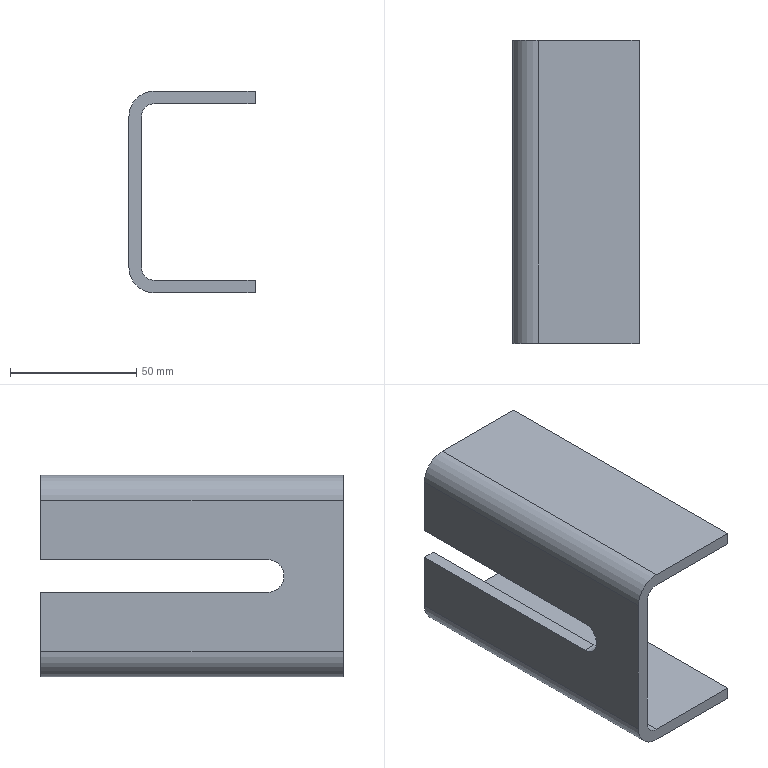Part | SolidWorks | features BaseBody 1 | 1 solid | 18 faces | box 50 x 120 x 80 mm | volume 91955 mm3 | plane 13 | cylinder 5 | commonest cylinder face diameters 10 x2 20 x2 13 x1
STEP:
#1=CARTESIAN_POINT('',(-50.,120.,21.101));
#2=VERTEX_POINT('',#1);
#3=CARTESIAN_POINT('',(-50.,30.,21.101));
#4=VERTEX_POINT('',#3);
#5=CARTESIAN_POINT('',(-50.,60.,21.101));
#6=DIRECTION('',(0.,-1.,0.));
#7=VECTOR('',#6,1000.);
#8=LINE('',#5,#7);
#9=EDGE_CURVE('',#2,#4,#8,.T.);
#10=ORIENTED_EDGE('',*,*,#9,.T.);
#11=CARTESIAN_POINT('',(-50.,30.,8.101));
#12=VERTEX_POINT('',#11);
#13=CARTESIAN_POINT('',(-50.,30.,14.601));
#14=DIRECTION('',(1.,0.,0.));
#15=DIRECTION('',(0.,0.,-1.));
#16=AXIS2_PLACEMENT_3D('',#13,#14,#15);
#17=CIRCLE('',#16,6.5);
#18=EDGE_CURVE('',#4,#12,#17,.T.);
#19=ORIENTED_EDGE('',*,*,#18,.T.);
#20=CARTESIAN_POINT('',(-50.,120.,8.101));
#21=VERTEX_POINT('',#20);
#22=CARTESIAN_POINT('',(-50.,60.,8.101));
#23=DIRECTION('',(0.,1.,0.));
#24=VECTOR('',#23,1000.);
#25=LINE('',#22,#24);
#26=EDGE_CURVE('',#12,#21,#25,.T.);
#27=ORIENTED_EDGE('',*,*,#26,.T.);
#28=CARTESIAN_POINT('',(-50.,120.,-15.399));
#29=VERTEX_POINT('',#28);
#30=CARTESIAN_POINT('',(-50.,120.,14.601));
#31=DIRECTION('',(0.,0.,-1.));
#32=VECTOR('',#31,1000.);
#33=LINE('',#30,#32);
#34=EDGE_CURVE('',#21,#29,#33,.T.);
#35=ORIENTED_EDGE('',*,*,#34,.T.);
#36=CARTESIAN_POINT('',(-50.,0.,-15.399));
#37=VERTEX_POINT('',#36);
#38=CARTESIAN_POINT('',(-50.,60.,-15.399));
#39=DIRECTION('',(0.,-1.,0.));
#40=VECTOR('',#39,1000.);
#41=LINE('',#38,#40);
#42=EDGE_CURVE('',#29,#37,#41,.T.);
#43=ORIENTED_EDGE('',*,*,#42,.T.);
#44=CARTESIAN_POINT('',(-50.,0.,44.601));
#45=VERTEX_POINT('',#44);
#46=CARTESIAN_POINT('',(-50.,0.,14.601));
#47=DIRECTION('',(0.,0.,1.));
#48=VECTOR('',#47,1000.);
#49=LINE('',#46,#48);
#50=EDGE_CURVE('',#37,#45,#49,.T.);
#51=ORIENTED_EDGE('',*,*,#50,.T.);
#52=CARTESIAN_POINT('',(-50.,120.,44.601));
#53=VERTEX_POINT('',#52);
#54=CARTESIAN_POINT('',(-50.,60.,44.601));
#55=DIRECTION('',(0.,1.,0.));
#56=VECTOR('',#55,1000.);
#57=LINE('',#54,#56);
#58=EDGE_CURVE('',#45,#53,#57,.T.);
#59=ORIENTED_EDGE('',*,*,#58,.T.);
#60=CARTESIAN_POINT('',(-50.,120.,14.601));
#61=DIRECTION('',(0.,0.,-1.));
#62=VECTOR('',#61,1000.);
#63=LINE('',#60,#62);
#64=EDGE_CURVE('',#53,#2,#63,.T.);
#65=ORIENTED_EDGE('',*,*,#64,.T.);
#66=EDGE_LOOP('',(#10,#19,#27,#35,#43,#51,#59,#65));
#67=FACE_OUTER_BOUND('',#66,.T.);
#68=CARTESIAN_POINT('',(-50.,60.,14.601));
#69=DIRECTION('',(-1.,0.,0.));
#70=DIRECTION('',(0.,0.,1.));
#71=AXIS2_PLACEMENT_3D('',#68,#69,#70);
#72=PLANE('',#71);
#73=ADVANCED_FACE('',(#67),#72,.T.);
#74=CARTESIAN_POINT('',(-45.,30.,21.101));
#75=VERTEX_POINT('',#74);
#76=CARTESIAN_POINT('',(-50.,30.,21.101));
#77=DIRECTION('',(-1.,0.,0.));
#78=VECTOR('',#77,1000.);
#79=LINE('',#76,#78);
#80=EDGE_CURVE('',#75,#4,#79,.T.);
#81=ORIENTED_EDGE('',*,*,#80,.F.);
#82=CARTESIAN_POINT('',(-45.,30.,8.101));
#83=VERTEX_POINT('',#82);
#84=CARTESIAN_POINT('',(-45.,30.,14.601));
#85=DIRECTION('',(-1.,0.,0.));
#86=DIRECTION('',(0.,0.,-1.));
#87=AXIS2_PLACEMENT_3D('',#84,#85,#86);
#88=CIRCLE('',#87,6.5);
#89=EDGE_CURVE('',#83,#75,#88,.T.);
#90=ORIENTED_EDGE('',*,*,#89,.F.);
#91=CARTESIAN_POINT('',(-50.,30.,8.101));
#92=DIRECTION('',(1.,0.,0.));
#93=VECTOR('',#92,1000.);
#94=LINE('',#91,#93);
#95=EDGE_CURVE('',#12,#83,#94,.T.);
#96=ORIENTED_EDGE('',*,*,#95,.F.);
#97=ORIENTED_EDGE('',*,*,#18,.F.);
#98=EDGE_LOOP('',(#81,#90,#96,#97));
#99=FACE_OUTER_BOUND('',#98,.T.);
#100=CARTESIAN_POINT('',(-50.,30.,14.601));
#101=DIRECTION('',(1.,0.,0.));
#102=DIRECTION('',(0.,0.,-1.));
#103=AXIS2_PLACEMENT_3D('',#100,#101,#102);
#104=CYLINDRICAL_SURFACE('',#103,6.5);
#105=ADVANCED_FACE('',(#99),#104,.F.);
#106=CARTESIAN_POINT('',(-45.,120.,21.101));
#107=VERTEX_POINT('',#106);
#108=CARTESIAN_POINT('',(-50.,120.,21.101));
#109=DIRECTION('',(-1.,0.,0.));
#110=VECTOR('',#109,1000.);
#111=LINE('',#108,#110);
#112=EDGE_CURVE('',#107,#2,#111,.T.);
#113=ORIENTED_EDGE('',*,*,#112,.F.);
#114=CARTESIAN_POINT('',(-45.,120.,21.101));
#115=DIRECTION('',(0.,1.,0.));
#116=VECTOR('',#115,1000.);
#117=LINE('',#114,#116);
#118=EDGE_CURVE('',#75,#107,#117,.T.);
#119=ORIENTED_EDGE('',*,*,#118,.F.);
#120=ORIENTED_EDGE('',*,*,#80,.T.);
#121=ORIENTED_EDGE('',*,*,#9,.F.);
#122=EDGE_LOOP('',(#113,#119,#120,#121));
#123=FACE_OUTER_BOUND('',#122,.T.);
#124=CARTESIAN_POINT('',(-50.,120.,21.101));
#125=DIRECTION('',(0.,0.,1.));
#126=DIRECTION('',(0.,-1.,0.));
#127=AXIS2_PLACEMENT_3D('',#124,#125,#126);
#128=PLANE('',#127);
#129=ADVANCED_FACE('',(#123),#128,.F.);
#130=ORIENTED_EDGE('',*,*,#64,.F.);
#131=CARTESIAN_POINT('',(-40.,120.,54.601));
#132=VERTEX_POINT('',#131);
#133=CARTESIAN_POINT('',(-40.,120.,44.601));
#134=DIRECTION('',(0.,-1.,0.));
#135=DIRECTION('',(0.,0.,-1.));
#136=AXIS2_PLACEMENT_3D('',#133,#134,#135);
#137=CIRCLE('',#136,10.);
#138=EDGE_CURVE('',#132,#53,#137,.T.);
#139=ORIENTED_EDGE('',*,*,#138,.F.);
#140=CARTESIAN_POINT('',(0.,120.,54.601));
#141=VERTEX_POINT('',#140);
#142=CARTESIAN_POINT('',(-81.31,120.,54.601));
#143=DIRECTION('',(-1.,0.,0.));
#144=VECTOR('',#143,1000.);
#145=LINE('',#142,#144);
#146=EDGE_CURVE('',#141,#132,#145,.T.);
#147=ORIENTED_EDGE('',*,*,#146,.F.);
#148=CARTESIAN_POINT('',(0.,120.,49.601));
#149=VERTEX_POINT('',#148);
#150=CARTESIAN_POINT('',(0.,120.,49.601));
#151=DIRECTION('',(0.,0.,-1.));
#152=VECTOR('',#151,1000.);
#153=LINE('',#150,#152);
#154=EDGE_CURVE('',#141,#149,#153,.T.);
#155=ORIENTED_EDGE('',*,*,#154,.T.);
#156=CARTESIAN_POINT('',(-40.,120.,49.601));
#157=VERTEX_POINT('',#156);
#158=CARTESIAN_POINT('',(-40.,120.,49.601));
#159=DIRECTION('',(-1.,0.,0.));
#160=VECTOR('',#159,1000.);
#161=LINE('',#158,#160);
#162=EDGE_CURVE('',#149,#157,#161,.T.);
#163=ORIENTED_EDGE('',*,*,#162,.T.);
#164=CARTESIAN_POINT('',(-45.,120.,44.601));
#165=VERTEX_POINT('',#164);
#166=CARTESIAN_POINT('',(-40.,120.,44.601));
#167=DIRECTION('',(0.,-1.,0.));
#168=DIRECTION('',(0.,0.,-1.));
#169=AXIS2_PLACEMENT_3D('',#166,#167,#168);
#170=CIRCLE('',#169,5.);
#171=EDGE_CURVE('',#157,#165,#170,.T.);
#172=ORIENTED_EDGE('',*,*,#171,.T.);
#173=CARTESIAN_POINT('',(-45.,120.,55.911));
#174=DIRECTION('',(0.,0.,-1.));
#175=VECTOR('',#174,1000.);
#176=LINE('',#173,#175);
#177=EDGE_CURVE('',#165,#107,#176,.T.);
#178=ORIENTED_EDGE('',*,*,#177,.T.);
#179=ORIENTED_EDGE('',*,*,#112,.T.);
#180=EDGE_LOOP('',(#130,#139,#147,#155,#163,#172,#178,#179));
#181=FACE_OUTER_BOUND('',#180,.T.);
#182=CARTESIAN_POINT('',(-45.,120.,55.911));
#183=DIRECTION('',(0.,1.,0.));
#184=DIRECTION('',(0.,0.,1.));
#185=AXIS2_PLACEMENT_3D('',#182,#183,#184);
#186=PLANE('',#185);
#187=ADVANCED_FACE('',(#181),#186,.T.);
#188=CARTESIAN_POINT('',(-40.,0.,54.601));
#189=VERTEX_POINT('',#188);
#190=CARTESIAN_POINT('',(-40.,60.,54.601));
#191=DIRECTION('',(0.,1.,0.));
#192=VECTOR('',#191,1000.);
#193=LINE('',#190,#192);
#194=EDGE_CURVE('',#189,#132,#193,.T.);
#195=ORIENTED_EDGE('',*,*,#194,.T.);
#196=ORIENTED_EDGE('',*,*,#138,.T.);
#197=ORIENTED_EDGE('',*,*,#58,.F.);
#198=CARTESIAN_POINT('',(-40.,0.,44.601));
#199=DIRECTION('',(0.,1.,0.));
#200=DIRECTION('',(0.,0.,-1.));
#201=AXIS2_PLACEMENT_3D('',#198,#199,#200);
#202=CIRCLE('',#201,10.);
#203=EDGE_CURVE('',#45,#189,#202,.T.);
#204=ORIENTED_EDGE('',*,*,#203,.T.);
#205=EDGE_LOOP('',(#195,#196,#197,#204));
#206=FACE_OUTER_BOUND('',#205,.T.);
#207=CARTESIAN_POINT('',(-40.,60.,44.601));
#208=DIRECTION('',(0.,-1.,0.));
#209=DIRECTION('',(0.,0.,-1.));
#210=AXIS2_PLACEMENT_3D('',#207,#208,#209);
#211=CYLINDRICAL_SURFACE('',#210,10.);
#212=ADVANCED_FACE('',(#206),#211,.T.);
#213=CARTESIAN_POINT('',(-45.,0.,-15.399));
#214=VERTEX_POINT('',#213);
#215=CARTESIAN_POINT('',(-45.,0.,44.601));
#216=VERTEX_POINT('',#215);
#217=CARTESIAN_POINT('',(-45.,0.,-26.709));
#218=DIRECTION('',(0.,0.,1.));
#219=VECTOR('',#218,1000.);
#220=LINE('',#217,#219);
#221=EDGE_CURVE('',#214,#216,#220,.T.);
#222=ORIENTED_EDGE('',*,*,#221,.T.);
#223=CARTESIAN_POINT('',(-40.,0.,49.601));
#224=VERTEX_POINT('',#223);
#225=CARTESIAN_POINT('',(-40.,0.,44.601));
#226=DIRECTION('',(0.,1.,0.));
#227=DIRECTION('',(0.,0.,-1.));
#228=AXIS2_PLACEMENT_3D('',#225,#226,#227);
#229=CIRCLE('',#228,5.);
#230=EDGE_CURVE('',#216,#224,#229,.T.);
#231=ORIENTED_EDGE('',*,*,#230,.T.);
#232=CARTESIAN_POINT('',(0.,0.,49.601));
#233=VERTEX_POINT('',#232);
#234=CARTESIAN_POINT('',(-122.619,0.,49.601));
#235=DIRECTION('',(1.,0.,0.));
#236=VECTOR('',#235,1000.);
#237=LINE('',#234,#236);
#238=EDGE_CURVE('',#224,#233,#237,.T.);
#239=ORIENTED_EDGE('',*,*,#238,.T.);
#240=CARTESIAN_POINT('',(0.,0.,54.601));
#241=VERTEX_POINT('',#240);
#242=CARTESIAN_POINT('',(0.,0.,49.601));
#243=DIRECTION('',(0.,0.,-1.));
#244=VECTOR('',#243,1000.);
#245=LINE('',#242,#244);
#246=EDGE_CURVE('',#241,#233,#245,.T.);
#247=ORIENTED_EDGE('',*,*,#246,.F.);
#248=CARTESIAN_POINT('',(-81.31,0.,54.601));
#249=DIRECTION('',(1.,0.,0.));
#250=VECTOR('',#249,1000.);
#251=LINE('',#248,#250);
#252=EDGE_CURVE('',#189,#241,#251,.T.);
#253=ORIENTED_EDGE('',*,*,#252,.F.);
#254=ORIENTED_EDGE('',*,*,#203,.F.);
#255=ORIENTED_EDGE('',*,*,#50,.F.);
#256=CARTESIAN_POINT('',(-40.,0.,-25.399));
#257=VERTEX_POINT('',#256);
#258=CARTESIAN_POINT('',(-40.,0.,-15.399));
#259=DIRECTION('',(0.,1.,0.));
#260=DIRECTION('',(0.,0.,-1.));
#261=AXIS2_PLACEMENT_3D('',#258,#259,#260);
#262=CIRCLE('',#261,10.);
#263=EDGE_CURVE('',#257,#37,#262,.T.);
#264=ORIENTED_EDGE('',*,*,#263,.F.);
#265=CARTESIAN_POINT('',(0.,0.,-25.399));
#266=VERTEX_POINT('',#265);
#267=CARTESIAN_POINT('',(-81.31,0.,-25.399));
#268=DIRECTION('',(-1.,0.,0.));
#269=VECTOR('',#268,1000.);
#270=LINE('',#267,#269);
#271=EDGE_CURVE('',#266,#257,#270,.T.);
#272=ORIENTED_EDGE('',*,*,#271,.F.);
#273=CARTESIAN_POINT('',(0.,0.,-20.399));
#274=VERTEX_POINT('',#273);
#275=CARTESIAN_POINT('',(0.,0.,-20.399));
#276=DIRECTION('',(0.,0.,1.));
#277=VECTOR('',#276,1000.);
#278=LINE('',#275,#277);
#279=EDGE_CURVE('',#266,#274,#278,.T.);
#280=ORIENTED_EDGE('',*,*,#279,.T.);
#281=CARTESIAN_POINT('',(-40.,0.,-20.399));
#282=VERTEX_POINT('',#281);
#283=CARTESIAN_POINT('',(-40.,0.,-20.399));
#284=DIRECTION('',(-1.,0.,0.));
#285=VECTOR('',#284,1000.);
#286=LINE('',#283,#285);
#287=EDGE_CURVE('',#274,#282,#286,.T.);
#288=ORIENTED_EDGE('',*,*,#287,.T.);
#289=CARTESIAN_POINT('',(-40.,0.,-15.399));
#290=DIRECTION('',(0.,1.,0.));
#291=DIRECTION('',(0.,0.,-1.));
#292=AXIS2_PLACEMENT_3D('',#289,#290,#291);
#293=CIRCLE('',#292,5.);
#294=EDGE_CURVE('',#282,#214,#293,.T.);
#295=ORIENTED_EDGE('',*,*,#294,.T.);
#296=EDGE_LOOP('',(#222,#231,#239,#247,#253,#254,#255,#264,#272,#280,#288,#295));
#297=FACE_OUTER_BOUND('',#296,.T.);
#298=CARTESIAN_POINT('',(-45.,0.,-26.709));
#299=DIRECTION('',(0.,-1.,0.));
#300=DIRECTION('',(0.,0.,-1.));
#301=AXIS2_PLACEMENT_3D('',#298,#299,#300);
#302=PLANE('',#301);
#303=ADVANCED_FACE('',(#297),#302,.T.);
#304=ORIENTED_EDGE('',*,*,#42,.F.);
#305=CARTESIAN_POINT('',(-40.,120.,-25.399));
#306=VERTEX_POINT('',#305);
#307=CARTESIAN_POINT('',(-40.,120.,-15.399));
#308=DIRECTION('',(0.,-1.,0.));
#309=DIRECTION('',(0.,0.,-1.));
#310=AXIS2_PLACEMENT_3D('',#307,#308,#309);
#311=CIRCLE('',#310,10.);
#312=EDGE_CURVE('',#29,#306,#311,.T.);
#313=ORIENTED_EDGE('',*,*,#312,.T.);
#314=CARTESIAN_POINT('',(-40.,60.,-25.399));
#315=DIRECTION('',(0.,-1.,0.));
#316=VECTOR('',#315,1000.);
#317=LINE('',#314,#316);
#318=EDGE_CURVE('',#306,#257,#317,.T.);
#319=ORIENTED_EDGE('',*,*,#318,.T.);
#320=ORIENTED_EDGE('',*,*,#263,.T.);
#321=EDGE_LOOP('',(#304,#313,#319,#320));
#322=FACE_OUTER_BOUND('',#321,.T.);
#323=CARTESIAN_POINT('',(-40.,60.,-15.399));
#324=DIRECTION('',(0.,-1.,0.));
#325=DIRECTION('',(0.,0.,-1.));
#326=AXIS2_PLACEMENT_3D('',#323,#324,#325);
#327=CYLINDRICAL_SURFACE('',#326,10.);
#328=ADVANCED_FACE('',(#322),#327,.T.);
#329=CARTESIAN_POINT('',(-45.,120.,8.101));
#330=VERTEX_POINT('',#329);
#331=CARTESIAN_POINT('',(-45.,120.,-15.399));
#332=VERTEX_POINT('',#331);
#333=CARTESIAN_POINT('',(-45.,120.,55.911));
#334=DIRECTION('',(0.,0.,-1.));
#335=VECTOR('',#334,1000.);
#336=LINE('',#333,#335);
#337=EDGE_CURVE('',#330,#332,#336,.T.);
#338=ORIENTED_EDGE('',*,*,#337,.T.);
#339=CARTESIAN_POINT('',(-40.,120.,-20.399));
#340=VERTEX_POINT('',#339);
#341=CARTESIAN_POINT('',(-40.,120.,-15.399));
#342=DIRECTION('',(0.,-1.,0.));
#343=DIRECTION('',(0.,0.,-1.));
#344=AXIS2_PLACEMENT_3D('',#341,#342,#343);
#345=CIRCLE('',#344,5.);
#346=EDGE_CURVE('',#332,#340,#345,.T.);
#347=ORIENTED_EDGE('',*,*,#346,.T.);
#348=CARTESIAN_POINT('',(0.,120.,-20.399));
#349=VERTEX_POINT('',#348);
#350=CARTESIAN_POINT('',(-122.619,120.,-20.399));
#351=DIRECTION('',(1.,0.,0.));
#352=VECTOR('',#351,1000.);
#353=LINE('',#350,#352);
#354=EDGE_CURVE('',#340,#349,#353,.T.);
#355=ORIENTED_EDGE('',*,*,#354,.T.);
#356=CARTESIAN_POINT('',(0.,120.,-25.399));
#357=VERTEX_POINT('',#356);
#358=CARTESIAN_POINT('',(0.,120.,-20.399));
#359=DIRECTION('',(0.,0.,-1.));
#360=VECTOR('',#359,1000.);
#361=LINE('',#358,#360);
#362=EDGE_CURVE('',#349,#357,#361,.T.);
#363=ORIENTED_EDGE('',*,*,#362,.T.);
#364=CARTESIAN_POINT('',(-81.31,120.,-25.399));
#365=DIRECTION('',(1.,0.,0.));
#366=VECTOR('',#365,1000.);
#367=LINE('',#364,#366);
#368=EDGE_CURVE('',#306,#357,#367,.T.);
#369=ORIENTED_EDGE('',*,*,#368,.F.);
#370=ORIENTED_EDGE('',*,*,#312,.F.);
#371=ORIENTED_EDGE('',*,*,#34,.F.);
#372=CARTESIAN_POINT('',(-45.,120.,8.101));
#373=DIRECTION('',(1.,0.,0.));
#374=VECTOR('',#373,1000.);
#375=LINE('',#372,#374);
#376=EDGE_CURVE('',#21,#330,#375,.T.);
#377=ORIENTED_EDGE('',*,*,#376,.T.);
#378=EDGE_LOOP('',(#338,#347,#355,#363,#369,#370,#371,#377));
#379=FACE_OUTER_BOUND('',#378,.T.);
#380=CARTESIAN_POINT('',(-45.,120.,55.911));
#381=DIRECTION('',(0.,1.,0.));
#382=DIRECTION('',(0.,0.,1.));
#383=AXIS2_PLACEMENT_3D('',#380,#381,#382);
#384=PLANE('',#383);
#385=ADVANCED_FACE('',(#379),#384,.T.);
#386=ORIENTED_EDGE('',*,*,#95,.T.);
#387=CARTESIAN_POINT('',(-45.,30.,8.101));
#388=DIRECTION('',(0.,-1.,0.));
#389=VECTOR('',#388,1000.);
#390=LINE('',#387,#389);
#391=EDGE_CURVE('',#330,#83,#390,.T.);
#392=ORIENTED_EDGE('',*,*,#391,.F.);
#393=ORIENTED_EDGE('',*,*,#376,.F.);
#394=ORIENTED_EDGE('',*,*,#26,.F.);
#395=EDGE_LOOP('',(#386,#392,#393,#394));
#396=FACE_OUTER_BOUND('',#395,.T.);
#397=CARTESIAN_POINT('',(-50.,30.,8.101));
#398=DIRECTION('',(0.,0.,-1.));
#399=DIRECTION('',(0.,1.,0.));
#400=AXIS2_PLACEMENT_3D('',#397,#398,#399);
#401=PLANE('',#400);
#402=ADVANCED_FACE('',(#396),#401,.F.);
#403=ORIENTED_EDGE('',*,*,#89,.T.);
#404=ORIENTED_EDGE('',*,*,#118,.T.);
#405=ORIENTED_EDGE('',*,*,#177,.F.);
#406=CARTESIAN_POINT('',(-45.,60.,44.601));
#407=DIRECTION('',(0.,1.,0.));
#408=VECTOR('',#407,1000.);
#409=LINE('',#406,#408);
#410=EDGE_CURVE('',#216,#165,#409,.T.);
#411=ORIENTED_EDGE('',*,*,#410,.F.);
#412=ORIENTED_EDGE('',*,*,#221,.F.);
#413=CARTESIAN_POINT('',(-45.,60.,-15.399));
#414=DIRECTION('',(0.,-1.,0.));
#415=VECTOR('',#414,1000.);
#416=LINE('',#413,#415);
#417=EDGE_CURVE('',#332,#214,#416,.T.);
#418=ORIENTED_EDGE('',*,*,#417,.F.);
#419=ORIENTED_EDGE('',*,*,#337,.F.);
#420=ORIENTED_EDGE('',*,*,#391,.T.);
#421=EDGE_LOOP('',(#403,#404,#405,#411,#412,#418,#419,#420));
#422=FACE_OUTER_BOUND('',#421,.T.);
#423=CARTESIAN_POINT('',(-45.,60.,14.601));
#424=DIRECTION('',(-1.,0.,0.));
#425=DIRECTION('',(0.,0.,1.));
#426=AXIS2_PLACEMENT_3D('',#423,#424,#425);
#427=PLANE('',#426);
#428=ADVANCED_FACE('',(#422),#427,.F.);
#429=CARTESIAN_POINT('',(0.,60.,54.601));
#430=DIRECTION('',(0.,1.,0.));
#431=VECTOR('',#430,1000.);
#432=LINE('',#429,#431);
#433=EDGE_CURVE('',#241,#141,#432,.T.);
#434=ORIENTED_EDGE('',*,*,#433,.T.);
#435=ORIENTED_EDGE('',*,*,#146,.T.);
#436=ORIENTED_EDGE('',*,*,#194,.F.);
#437=ORIENTED_EDGE('',*,*,#252,.T.);
#438=EDGE_LOOP('',(#434,#435,#436,#437));
#439=FACE_OUTER_BOUND('',#438,.T.);
#440=CARTESIAN_POINT('',(-81.31,60.,54.601));
#441=DIRECTION('',(0.,0.,1.));
#442=DIRECTION('',(1.,0.,0.));
#443=AXIS2_PLACEMENT_3D('',#440,#441,#442);
#444=PLANE('',#443);
#445=ADVANCED_FACE('',(#439),#444,.T.);
#446=CARTESIAN_POINT('',(0.,60.,-25.399));
#447=DIRECTION('',(0.,-1.,0.));
#448=VECTOR('',#447,1000.);
#449=LINE('',#446,#448);
#450=EDGE_CURVE('',#357,#266,#449,.T.);
#451=ORIENTED_EDGE('',*,*,#450,.T.);
#452=ORIENTED_EDGE('',*,*,#271,.T.);
#453=ORIENTED_EDGE('',*,*,#318,.F.);
#454=ORIENTED_EDGE('',*,*,#368,.T.);
#455=EDGE_LOOP('',(#451,#452,#453,#454));
#456=FACE_OUTER_BOUND('',#455,.T.);
#457=CARTESIAN_POINT('',(-81.31,60.,-25.399));
#458=DIRECTION('',(0.,0.,-1.));
#459=DIRECTION('',(-1.,0.,0.));
#460=AXIS2_PLACEMENT_3D('',#457,#458,#459);
#461=PLANE('',#460);
#462=ADVANCED_FACE('',(#456),#461,.T.);
#463=ORIENTED_EDGE('',*,*,#171,.F.);
#464=CARTESIAN_POINT('',(-40.,60.,49.601));
#465=DIRECTION('',(0.,1.,0.));
#466=VECTOR('',#465,1000.);
#467=LINE('',#464,#466);
#468=EDGE_CURVE('',#224,#157,#467,.T.);
#469=ORIENTED_EDGE('',*,*,#468,.F.);
#470=ORIENTED_EDGE('',*,*,#230,.F.);
#471=ORIENTED_EDGE('',*,*,#410,.T.);
#472=EDGE_LOOP('',(#463,#469,#470,#471));
#473=FACE_OUTER_BOUND('',#472,.T.);
#474=CARTESIAN_POINT('',(-40.,60.,44.601));
#475=DIRECTION('',(0.,-1.,0.));
#476=DIRECTION('',(0.,0.,-1.));
#477=AXIS2_PLACEMENT_3D('',#474,#475,#476);
#478=CYLINDRICAL_SURFACE('',#477,5.);
#479=ADVANCED_FACE('',(#473),#478,.F.);
#480=ORIENTED_EDGE('',*,*,#346,.F.);
#481=ORIENTED_EDGE('',*,*,#417,.T.);
#482=ORIENTED_EDGE('',*,*,#294,.F.);
#483=CARTESIAN_POINT('',(-40.,60.,-20.399));
#484=DIRECTION('',(0.,-1.,0.));
#485=VECTOR('',#484,1000.);
#486=LINE('',#483,#485);
#487=EDGE_CURVE('',#340,#282,#486,.T.);
#488=ORIENTED_EDGE('',*,*,#487,.F.);
#489=EDGE_LOOP('',(#480,#481,#482,#488));
#490=FACE_OUTER_BOUND('',#489,.T.);
#491=CARTESIAN_POINT('',(-40.,60.,-15.399));
#492=DIRECTION('',(0.,-1.,0.));
#493=DIRECTION('',(0.,0.,-1.));
#494=AXIS2_PLACEMENT_3D('',#491,#492,#493);
#495=CYLINDRICAL_SURFACE('',#494,5.);
#496=ADVANCED_FACE('',(#490),#495,.F.);
#497=CARTESIAN_POINT('',(0.,120.,49.601));
#498=DIRECTION('',(0.,1.,0.));
#499=VECTOR('',#498,1000.);
#500=LINE('',#497,#499);
#501=EDGE_CURVE('',#233,#149,#500,.T.);
#502=ORIENTED_EDGE('',*,*,#501,.T.);
#503=ORIENTED_EDGE('',*,*,#154,.F.);
#504=ORIENTED_EDGE('',*,*,#433,.F.);
#505=ORIENTED_EDGE('',*,*,#246,.T.);
#506=EDGE_LOOP('',(#502,#503,#504,#505));
#507=FACE_OUTER_BOUND('',#506,.T.);
#508=CARTESIAN_POINT('',(0.,120.,49.601));
#509=DIRECTION('',(1.,0.,0.));
#510=DIRECTION('',(0.,0.,-1.));
#511=AXIS2_PLACEMENT_3D('',#508,#509,#510);
#512=PLANE('',#511);
#513=ADVANCED_FACE('',(#507),#512,.T.);
#514=CARTESIAN_POINT('',(0.,0.,-20.399));
#515=DIRECTION('',(0.,-1.,0.));
#516=VECTOR('',#515,1000.);
#517=LINE('',#514,#516);
#518=EDGE_CURVE('',#349,#274,#517,.T.);
#519=ORIENTED_EDGE('',*,*,#518,.T.);
#520=ORIENTED_EDGE('',*,*,#279,.F.);
#521=ORIENTED_EDGE('',*,*,#450,.F.);
#522=ORIENTED_EDGE('',*,*,#362,.F.);
#523=EDGE_LOOP('',(#519,#520,#521,#522));
#524=FACE_OUTER_BOUND('',#523,.T.);
#525=CARTESIAN_POINT('',(0.,0.,-20.399));
#526=DIRECTION('',(1.,0.,0.));
#527=DIRECTION('',(0.,0.,-1.));
#528=AXIS2_PLACEMENT_3D('',#525,#526,#527);
#529=PLANE('',#528);
#530=ADVANCED_FACE('',(#524),#529,.T.);
#531=ORIENTED_EDGE('',*,*,#162,.F.);
#532=ORIENTED_EDGE('',*,*,#501,.F.);
#533=ORIENTED_EDGE('',*,*,#238,.F.);
#534=ORIENTED_EDGE('',*,*,#468,.T.);
#535=EDGE_LOOP('',(#531,#532,#533,#534));
#536=FACE_OUTER_BOUND('',#535,.T.);
#537=CARTESIAN_POINT('',(-81.31,60.,49.601));
#538=DIRECTION('',(0.,0.,1.));
#539=DIRECTION('',(1.,0.,0.));
#540=AXIS2_PLACEMENT_3D('',#537,#538,#539);
#541=PLANE('',#540);
#542=ADVANCED_FACE('',(#536),#541,.F.);
#543=ORIENTED_EDGE('',*,*,#287,.F.);
#544=ORIENTED_EDGE('',*,*,#518,.F.);
#545=ORIENTED_EDGE('',*,*,#354,.F.);
#546=ORIENTED_EDGE('',*,*,#487,.T.);
#547=EDGE_LOOP('',(#543,#544,#545,#546));
#548=FACE_OUTER_BOUND('',#547,.T.);
#549=CARTESIAN_POINT('',(-81.31,60.,-20.399));
#550=DIRECTION('',(0.,0.,-1.));
#551=DIRECTION('',(-1.,0.,0.));
#552=AXIS2_PLACEMENT_3D('',#549,#550,#551);
#553=PLANE('',#552);
#554=ADVANCED_FACE('',(#548),#553,.F.);
#555=CLOSED_SHELL('',(#73,#105,#129,#187,#212,#303,#328,#385,#402,#428,#445,#462,#479,#496,#513,#530,#542,#554));
#556=MANIFOLD_SOLID_BREP('',#555);
#557=CARTESIAN_POINT('',(0.,0.,0.));
#558=DIRECTION('',(0.,0.,1.));
#559=DIRECTION('',(1.,0.,0.));
#560=AXIS2_PLACEMENT_3D('',#557,#558,#559);
#561=(LENGTH_UNIT()NAMED_UNIT(*)SI_UNIT(.MILLI.,.METRE.));
#562=UNCERTAINTY_MEASURE_WITH_UNIT(LENGTH_MEASURE(0.00001),#561,'','');
#563=(NAMED_UNIT(*)PLANE_ANGLE_UNIT()SI_UNIT($,.RADIAN.));
#564=(NAMED_UNIT(*)SI_UNIT($,.STERADIAN.)SOLID_ANGLE_UNIT());
#565=(GEOMETRIC_REPRESENTATION_CONTEXT(3)GLOBAL_UNCERTAINTY_ASSIGNED_CONTEXT((#562))GLOBAL_UNIT_ASSIGNED_CONTEXT((#561,#563,#564))REPRESENTATION_CONTEXT('',''));
#566=ADVANCED_BREP_SHAPE_REPRESENTATION('',(#556,#560),#565);